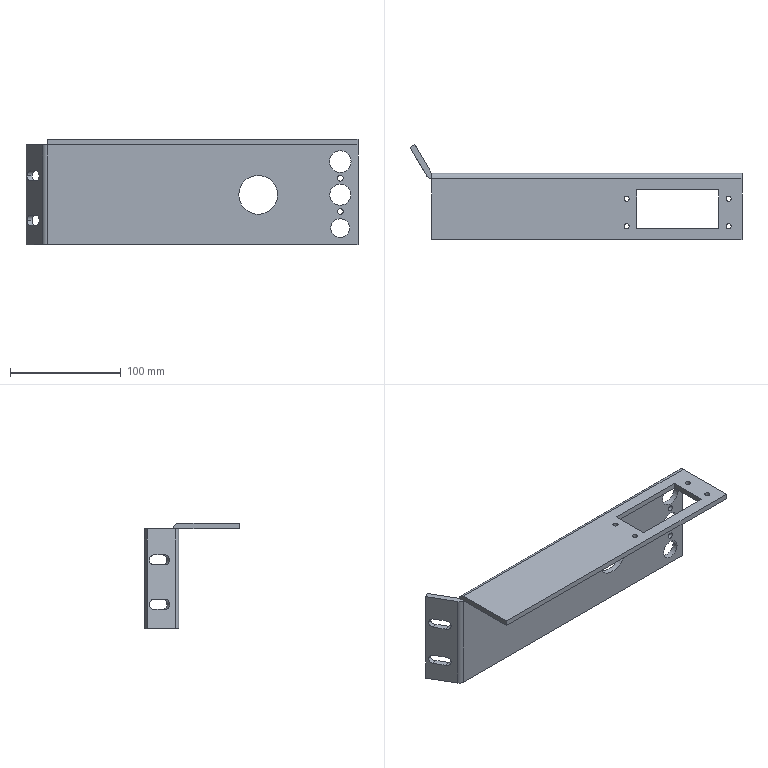Part | STEP file | Cable Chain Bracket_Default SM-FLAT-PATTERN | 1 solid | 50 faces | box 299.33 x 85.981 x 95.1 mm | volume 199185 mm3 | cylinder 30 | plane 20 | commonest cylinder face diameters 4.602 x8 9 x6 5.2 x4 0.2 x2 10.2 x2 16.983 x2